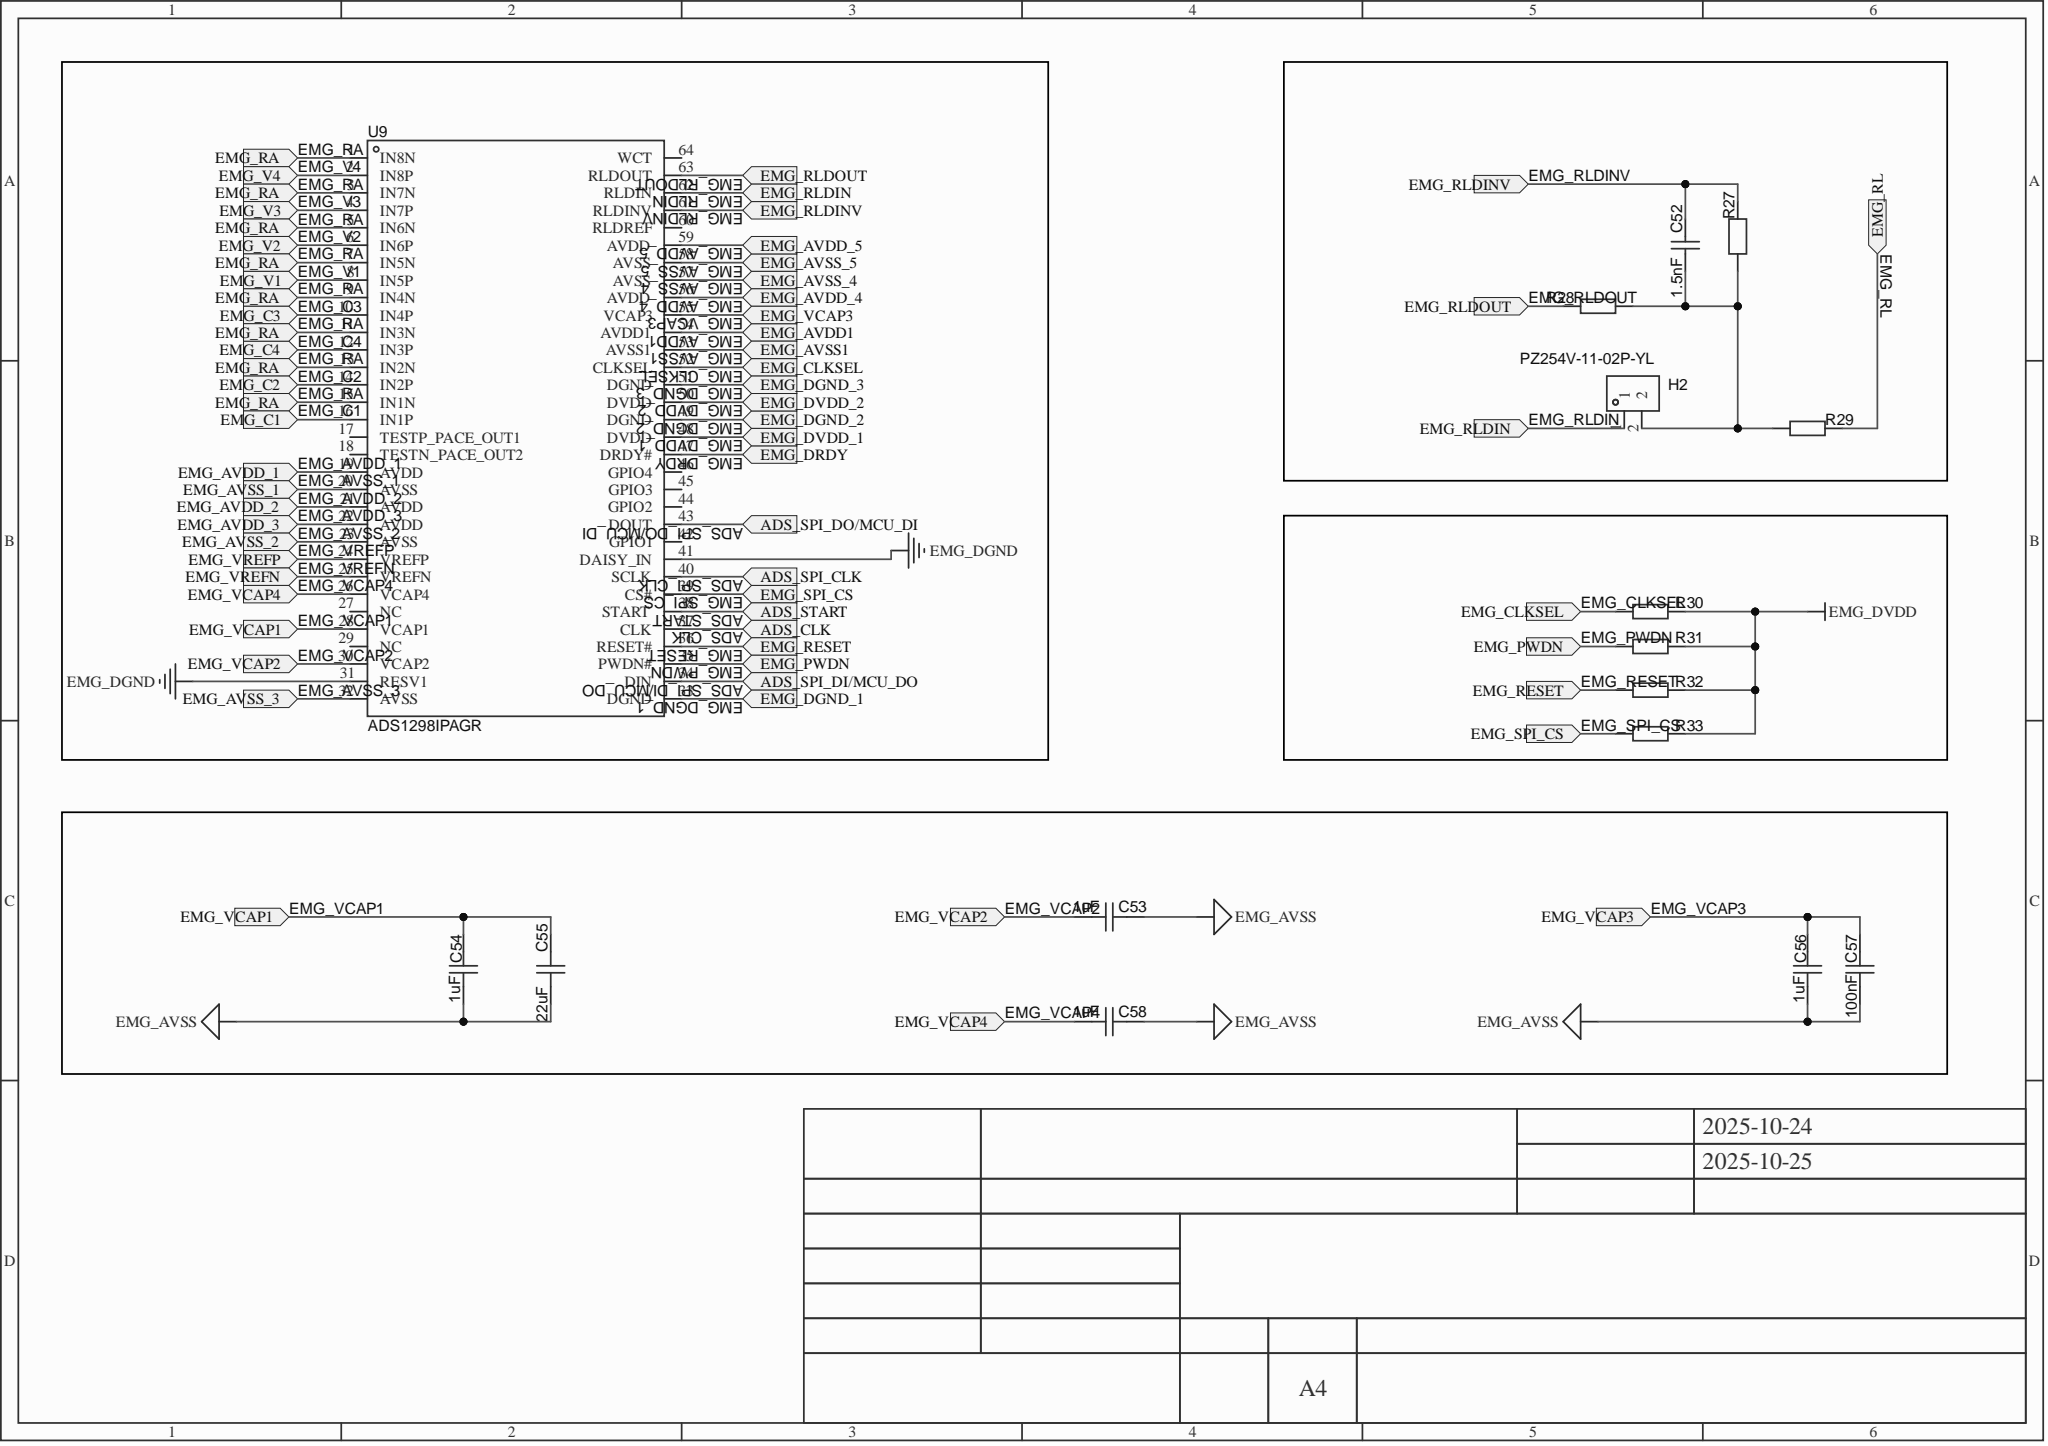Circuit board | Altium Designer | 211 parts | 126 nets | one sheet of the schematic
Parts on this sheet (reference | value | footprint):
C52 | 1.5nF | C0402
C53 | 1uF | C0402
C54 | 1uF | C0402
C55 | 22uF | C1206
C56 | 1uF | C0402
C57 | 100nF | C0402
C58 | 1uF | C0402
H2 | PZ254V-11-02P-YL | HDR-TH_2P-P2.54-V-M
R27 | R0402
R28 | R0402
R29 | R0402
R30 | R0402
R31 | R0402
R32 | R0402
R33 | R0402
U9 | ADS1298IPAGR | TQFP-64_L10.0-W10.0-P0.50-LS12.0-BL
Nets of these parts (net: part-pin ...):
NetC52_1: C52-1 H2-2 R27-2 R28-2 R29-1
EMG_VREFP: U9-24
EMG_VCAP4: C58-1 U9-26
EMG_VCAP3: C56-2 C57-2 U9-55
EMG_VCAP2: C53-1 U9-30
EMG_VCAP1: C54-2 C55-2 U9-28
EMG_V4: U9-2
EMG_V3: U9-4
EMG_V2: U9-6
EMG_V1: U9-8
EMG_SPI_CS: R33-1 U9-39
EMG_RLDOUT: R28-1 U9-63
EMG_RLDINV: C52-2 R27-1 U9-61
EMG_RLDIN: H2-1 U9-62
EMG_RL: R29-2
EMG_RESET: R32-1 U9-36
EMG_RA: U9-1 U9-3 U9-5 U9-7 U9-9 U9-11 U9-13 U9-15
EMG_PWDN: R31-1 U9-35
EMG_DVDD_1: R30-2 R31-2 R32-2 R33-2 U9-48 U9-50
EMG_DRDY: U9-47
EMG_DGND_1: U9-31 U9-33 U9-41 U9-49 U9-51
EMG_CLKSEL: R30-1 U9-52
EMG_C4: U9-12
EMG_C3: U9-10
EMG_C2: U9-14
EMG_C1: U9-16
EMG_AVSS1: C53-2 C54-1 C55-1 C56-1 C57-1 C58-2 U9-20 U9-23 U9-25 U9-32 U9-53 U9-57 U9-58
EMG_AVDD1: U9-19 U9-21 U9-22 U9-54 U9-56 U9-59
ADS_START: U9-38
ADS_SPI_DO/MCU_DI: U9-43
ADS_SPI_DI/MCU_DO: U9-34
ADS_SPI_CLK: U9-40
ADS_CLK: U9-37